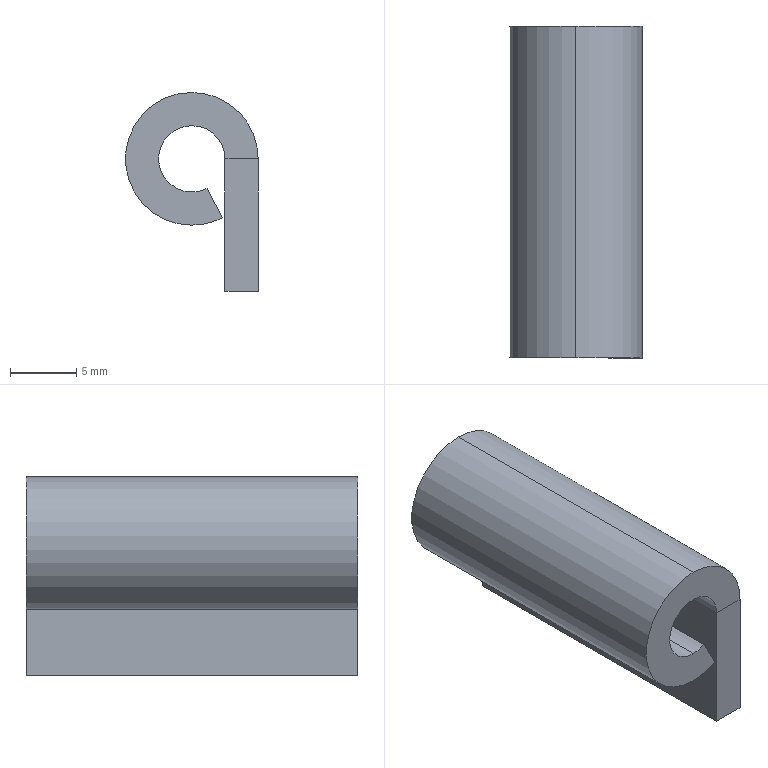Part | SolidWorks | features FlatPattern 1, SMBaseFlange 1, SheetMetal 1 | 1 solid | 14 faces | box 10 x 25 x 15 mm | volume 1841 mm3 | plane 8 | cylinder 6 | commonest cylinder face diameters 5 x3 10 x3
STEP:
#1=CARTESIAN_POINT('',(0.,25.,10.));
#2=VERTEX_POINT('',#1);
#3=CARTESIAN_POINT('',(-5.,25.,15.));
#4=VERTEX_POINT('',#3);
#5=CARTESIAN_POINT('',(-5.,25.,10.));
#6=DIRECTION('',(0.,-1.,0.));
#7=DIRECTION('',(0.,0.,-1.));
#8=AXIS2_PLACEMENT_3D('',#5,#6,#7);
#9=CIRCLE('',#8,5.);
#10=EDGE_CURVE('',#2,#4,#9,.T.);
#11=ORIENTED_EDGE('',*,*,#10,.T.);
#12=CARTESIAN_POINT('',(-5.,0.,15.));
#13=VERTEX_POINT('',#12);
#14=CARTESIAN_POINT('',(-5.,25.,15.));
#15=DIRECTION('',(0.,-1.,0.));
#16=VECTOR('',#15,1000.);
#17=LINE('',#14,#16);
#18=EDGE_CURVE('',#4,#13,#17,.T.);
#19=ORIENTED_EDGE('',*,*,#18,.T.);
#20=CARTESIAN_POINT('',(0.,0.,10.));
#21=VERTEX_POINT('',#20);
#22=CARTESIAN_POINT('',(-5.,0.,10.));
#23=DIRECTION('',(0.,-1.,0.));
#24=DIRECTION('',(0.,0.,-1.));
#25=AXIS2_PLACEMENT_3D('',#22,#23,#24);
#26=CIRCLE('',#25,5.);
#27=EDGE_CURVE('',#21,#13,#26,.T.);
#28=ORIENTED_EDGE('',*,*,#27,.F.);
#29=CARTESIAN_POINT('',(0.,25.,10.));
#30=DIRECTION('',(0.,-1.,0.));
#31=VECTOR('',#30,1000.);
#32=LINE('',#29,#31);
#33=EDGE_CURVE('',#2,#21,#32,.T.);
#34=ORIENTED_EDGE('',*,*,#33,.F.);
#35=EDGE_LOOP('',(#11,#19,#28,#34));
#36=FACE_OUTER_BOUND('',#35,.T.);
#37=CARTESIAN_POINT('',(-5.,25.,10.));
#38=DIRECTION('',(0.,-1.,0.));
#39=DIRECTION('',(0.,0.,-1.));
#40=AXIS2_PLACEMENT_3D('',#37,#38,#39);
#41=CYLINDRICAL_SURFACE('',#40,5.);
#42=ADVANCED_FACE('',(#36),#41,.T.);
#43=ORIENTED_EDGE('',*,*,#18,.F.);
#44=CARTESIAN_POINT('',(-5.,25.,5.));
#45=VERTEX_POINT('',#44);
#46=CARTESIAN_POINT('',(-5.,25.,10.));
#47=DIRECTION('',(0.,-1.,0.));
#48=DIRECTION('',(0.,0.,-1.));
#49=AXIS2_PLACEMENT_3D('',#46,#47,#48);
#50=CIRCLE('',#49,5.);
#51=EDGE_CURVE('',#4,#45,#50,.T.);
#52=ORIENTED_EDGE('',*,*,#51,.T.);
#53=CARTESIAN_POINT('',(-5.,0.,5.));
#54=VERTEX_POINT('',#53);
#55=CARTESIAN_POINT('',(-5.,25.,5.));
#56=DIRECTION('',(0.,-1.,0.));
#57=VECTOR('',#56,1000.);
#58=LINE('',#55,#57);
#59=EDGE_CURVE('',#45,#54,#58,.T.);
#60=ORIENTED_EDGE('',*,*,#59,.T.);
#61=CARTESIAN_POINT('',(-5.,0.,10.));
#62=DIRECTION('',(0.,-1.,0.));
#63=DIRECTION('',(0.,0.,-1.));
#64=AXIS2_PLACEMENT_3D('',#61,#62,#63);
#65=CIRCLE('',#64,5.);
#66=EDGE_CURVE('',#13,#54,#65,.T.);
#67=ORIENTED_EDGE('',*,*,#66,.F.);
#68=EDGE_LOOP('',(#43,#52,#60,#67));
#69=FACE_OUTER_BOUND('',#68,.T.);
#70=CARTESIAN_POINT('',(-5.,25.,10.));
#71=DIRECTION('',(0.,-1.,0.));
#72=DIRECTION('',(0.,0.,-1.));
#73=AXIS2_PLACEMENT_3D('',#70,#71,#72);
#74=CYLINDRICAL_SURFACE('',#73,5.);
#75=ADVANCED_FACE('',(#69),#74,.T.);
#76=CARTESIAN_POINT('',(-5.,25.,12.5));
#77=VERTEX_POINT('',#76);
#78=CARTESIAN_POINT('',(-5.,25.,7.5));
#79=VERTEX_POINT('',#78);
#80=CARTESIAN_POINT('',(-5.,25.,10.));
#81=DIRECTION('',(0.,-1.,0.));
#82=DIRECTION('',(1.,0.,0.));
#83=AXIS2_PLACEMENT_3D('',#80,#81,#82);
#84=CIRCLE('',#83,2.5);
#85=EDGE_CURVE('',#77,#79,#84,.T.);
#86=ORIENTED_EDGE('',*,*,#85,.F.);
#87=CARTESIAN_POINT('',(-5.,0.,12.5));
#88=VERTEX_POINT('',#87);
#89=CARTESIAN_POINT('',(-5.,25.,12.5));
#90=DIRECTION('',(0.,-1.,0.));
#91=VECTOR('',#90,1000.);
#92=LINE('',#89,#91);
#93=EDGE_CURVE('',#77,#88,#92,.T.);
#94=ORIENTED_EDGE('',*,*,#93,.T.);
#95=CARTESIAN_POINT('',(-5.,0.,7.5));
#96=VERTEX_POINT('',#95);
#97=CARTESIAN_POINT('',(-5.,0.,10.));
#98=DIRECTION('',(0.,-1.,0.));
#99=DIRECTION('',(1.,0.,0.));
#100=AXIS2_PLACEMENT_3D('',#97,#98,#99);
#101=CIRCLE('',#100,2.5);
#102=EDGE_CURVE('',#88,#96,#101,.T.);
#103=ORIENTED_EDGE('',*,*,#102,.T.);
#104=CARTESIAN_POINT('',(-5.,25.,7.5));
#105=DIRECTION('',(0.,-1.,0.));
#106=VECTOR('',#105,1000.);
#107=LINE('',#104,#106);
#108=EDGE_CURVE('',#79,#96,#107,.T.);
#109=ORIENTED_EDGE('',*,*,#108,.F.);
#110=EDGE_LOOP('',(#86,#94,#103,#109));
#111=FACE_OUTER_BOUND('',#110,.T.);
#112=CARTESIAN_POINT('',(-5.,25.,10.));
#113=DIRECTION('',(0.,-1.,0.));
#114=DIRECTION('',(0.,0.,-1.));
#115=AXIS2_PLACEMENT_3D('',#112,#113,#114);
#116=CYLINDRICAL_SURFACE('',#115,2.5);
#117=ADVANCED_FACE('',(#111),#116,.F.);
#118=CARTESIAN_POINT('',(-3.85,25.,7.78));
#119=VERTEX_POINT('',#118);
#120=CARTESIAN_POINT('',(-5.,25.,10.));
#121=DIRECTION('',(0.,-1.,0.));
#122=DIRECTION('',(1.,0.,0.));
#123=AXIS2_PLACEMENT_3D('',#120,#121,#122);
#124=CIRCLE('',#123,2.5);
#125=EDGE_CURVE('',#79,#119,#124,.T.);
#126=ORIENTED_EDGE('',*,*,#125,.F.);
#127=ORIENTED_EDGE('',*,*,#108,.T.);
#128=CARTESIAN_POINT('',(-3.85,0.,7.78));
#129=VERTEX_POINT('',#128);
#130=CARTESIAN_POINT('',(-5.,0.,10.));
#131=DIRECTION('',(0.,-1.,0.));
#132=DIRECTION('',(1.,0.,0.));
#133=AXIS2_PLACEMENT_3D('',#130,#131,#132);
#134=CIRCLE('',#133,2.5);
#135=EDGE_CURVE('',#96,#129,#134,.T.);
#136=ORIENTED_EDGE('',*,*,#135,.T.);
#137=CARTESIAN_POINT('',(-3.85,25.,7.78));
#138=DIRECTION('',(0.,-1.,0.));
#139=VECTOR('',#138,1000.);
#140=LINE('',#137,#139);
#141=EDGE_CURVE('',#119,#129,#140,.T.);
#142=ORIENTED_EDGE('',*,*,#141,.F.);
#143=EDGE_LOOP('',(#126,#127,#136,#142));
#144=FACE_OUTER_BOUND('',#143,.T.);
#145=CARTESIAN_POINT('',(-5.,25.,10.));
#146=DIRECTION('',(0.,-1.,0.));
#147=DIRECTION('',(0.,0.,-1.));
#148=AXIS2_PLACEMENT_3D('',#145,#146,#147);
#149=CYLINDRICAL_SURFACE('',#148,2.5);
#150=ADVANCED_FACE('',(#144),#149,.F.);
#151=CARTESIAN_POINT('',(-2.5,25.,10.));
#152=VERTEX_POINT('',#151);
#153=CARTESIAN_POINT('',(-2.5,25.,10.));
#154=DIRECTION('',(1.,0.,0.));
#155=VECTOR('',#154,1000.);
#156=LINE('',#153,#155);
#157=EDGE_CURVE('',#152,#2,#156,.T.);
#158=ORIENTED_EDGE('',*,*,#157,.F.);
#159=CARTESIAN_POINT('',(-5.,25.,10.));
#160=DIRECTION('',(0.,-1.,0.));
#161=DIRECTION('',(1.,0.,0.));
#162=AXIS2_PLACEMENT_3D('',#159,#160,#161);
#163=CIRCLE('',#162,2.5);
#164=EDGE_CURVE('',#152,#77,#163,.T.);
#165=ORIENTED_EDGE('',*,*,#164,.T.);
#166=ORIENTED_EDGE('',*,*,#85,.T.);
#167=ORIENTED_EDGE('',*,*,#125,.T.);
#168=CARTESIAN_POINT('',(-2.7,25.,5.56));
#169=VERTEX_POINT('',#168);
#170=CARTESIAN_POINT('',(-2.7,25.,5.56));
#171=DIRECTION('',(-0.46,0.,0.8879));
#172=VECTOR('',#171,1000.);
#173=LINE('',#170,#172);
#174=EDGE_CURVE('',#169,#119,#173,.T.);
#175=ORIENTED_EDGE('',*,*,#174,.F.);
#176=CARTESIAN_POINT('',(-5.,25.,10.));
#177=DIRECTION('',(0.,-1.,0.));
#178=DIRECTION('',(0.,0.,-1.));
#179=AXIS2_PLACEMENT_3D('',#176,#177,#178);
#180=CIRCLE('',#179,5.);
#181=EDGE_CURVE('',#45,#169,#180,.T.);
#182=ORIENTED_EDGE('',*,*,#181,.F.);
#183=ORIENTED_EDGE('',*,*,#51,.F.);
#184=ORIENTED_EDGE('',*,*,#10,.F.);
#185=EDGE_LOOP('',(#158,#165,#166,#167,#175,#182,#183,#184));
#186=FACE_OUTER_BOUND('',#185,.T.);
#187=CARTESIAN_POINT('',(-2.5,25.,10.));
#188=DIRECTION('',(0.,1.,0.));
#189=DIRECTION('',(0.,0.,1.));
#190=AXIS2_PLACEMENT_3D('',#187,#188,#189);
#191=PLANE('',#190);
#192=ADVANCED_FACE('',(#186),#191,.T.);
#193=CARTESIAN_POINT('',(-2.5,0.,10.));
#194=VERTEX_POINT('',#193);
#195=CARTESIAN_POINT('',(0.,0.,10.));
#196=DIRECTION('',(-1.,0.,0.));
#197=VECTOR('',#196,1000.);
#198=LINE('',#195,#197);
#199=EDGE_CURVE('',#21,#194,#198,.T.);
#200=ORIENTED_EDGE('',*,*,#199,.F.);
#201=ORIENTED_EDGE('',*,*,#27,.T.);
#202=ORIENTED_EDGE('',*,*,#66,.T.);
#203=CARTESIAN_POINT('',(-2.7,0.,5.56));
#204=VERTEX_POINT('',#203);
#205=CARTESIAN_POINT('',(-5.,0.,10.));
#206=DIRECTION('',(0.,-1.,0.));
#207=DIRECTION('',(0.,0.,-1.));
#208=AXIS2_PLACEMENT_3D('',#205,#206,#207);
#209=CIRCLE('',#208,5.);
#210=EDGE_CURVE('',#54,#204,#209,.T.);
#211=ORIENTED_EDGE('',*,*,#210,.T.);
#212=CARTESIAN_POINT('',(-2.7,0.,5.56));
#213=DIRECTION('',(-0.46,0.,0.8879));
#214=VECTOR('',#213,1000.);
#215=LINE('',#212,#214);
#216=EDGE_CURVE('',#204,#129,#215,.T.);
#217=ORIENTED_EDGE('',*,*,#216,.T.);
#218=ORIENTED_EDGE('',*,*,#135,.F.);
#219=ORIENTED_EDGE('',*,*,#102,.F.);
#220=CARTESIAN_POINT('',(-5.,0.,10.));
#221=DIRECTION('',(0.,-1.,0.));
#222=DIRECTION('',(1.,0.,0.));
#223=AXIS2_PLACEMENT_3D('',#220,#221,#222);
#224=CIRCLE('',#223,2.5);
#225=EDGE_CURVE('',#194,#88,#224,.T.);
#226=ORIENTED_EDGE('',*,*,#225,.F.);
#227=EDGE_LOOP('',(#200,#201,#202,#211,#217,#218,#219,#226));
#228=FACE_OUTER_BOUND('',#227,.T.);
#229=CARTESIAN_POINT('',(0.,0.,10.));
#230=DIRECTION('',(0.,-1.,0.));
#231=DIRECTION('',(0.,0.,-1.));
#232=AXIS2_PLACEMENT_3D('',#229,#230,#231);
#233=PLANE('',#232);
#234=ADVANCED_FACE('',(#228),#233,.T.);
#235=ORIENTED_EDGE('',*,*,#93,.F.);
#236=ORIENTED_EDGE('',*,*,#164,.F.);
#237=CARTESIAN_POINT('',(-2.5,25.,10.));
#238=DIRECTION('',(0.,-1.,0.));
#239=VECTOR('',#238,1000.);
#240=LINE('',#237,#239);
#241=EDGE_CURVE('',#152,#194,#240,.T.);
#242=ORIENTED_EDGE('',*,*,#241,.T.);
#243=ORIENTED_EDGE('',*,*,#225,.T.);
#244=EDGE_LOOP('',(#235,#236,#242,#243));
#245=FACE_OUTER_BOUND('',#244,.T.);
#246=CARTESIAN_POINT('',(-5.,25.,10.));
#247=DIRECTION('',(0.,-1.,0.));
#248=DIRECTION('',(0.,0.,-1.));
#249=AXIS2_PLACEMENT_3D('',#246,#247,#248);
#250=CYLINDRICAL_SURFACE('',#249,2.5);
#251=ADVANCED_FACE('',(#245),#250,.F.);
#252=ORIENTED_EDGE('',*,*,#216,.F.);
#253=CARTESIAN_POINT('',(-2.7,25.,5.56));
#254=DIRECTION('',(0.,-1.,0.));
#255=VECTOR('',#254,1000.);
#256=LINE('',#253,#255);
#257=EDGE_CURVE('',#169,#204,#256,.T.);
#258=ORIENTED_EDGE('',*,*,#257,.F.);
#259=ORIENTED_EDGE('',*,*,#174,.T.);
#260=ORIENTED_EDGE('',*,*,#141,.T.);
#261=EDGE_LOOP('',(#252,#258,#259,#260));
#262=FACE_OUTER_BOUND('',#261,.T.);
#263=CARTESIAN_POINT('',(-2.7,25.,5.56));
#264=DIRECTION('',(0.8879,0.,0.46));
#265=DIRECTION('',(0.46,0.,-0.8879));
#266=AXIS2_PLACEMENT_3D('',#263,#264,#265);
#267=PLANE('',#266);
#268=ADVANCED_FACE('',(#262),#267,.T.);
#269=ORIENTED_EDGE('',*,*,#59,.F.);
#270=ORIENTED_EDGE('',*,*,#181,.T.);
#271=ORIENTED_EDGE('',*,*,#257,.T.);
#272=ORIENTED_EDGE('',*,*,#210,.F.);
#273=EDGE_LOOP('',(#269,#270,#271,#272));
#274=FACE_OUTER_BOUND('',#273,.T.);
#275=CARTESIAN_POINT('',(-5.,25.,10.));
#276=DIRECTION('',(0.,-1.,0.));
#277=DIRECTION('',(0.,0.,-1.));
#278=AXIS2_PLACEMENT_3D('',#275,#276,#277);
#279=CYLINDRICAL_SURFACE('',#278,5.);
#280=ADVANCED_FACE('',(#274),#279,.T.);
#281=CARTESIAN_POINT('',(0.,0.,0.));
#282=VERTEX_POINT('',#281);
#283=CARTESIAN_POINT('',(0.,0.,0.));
#284=DIRECTION('',(0.,0.,1.));
#285=VECTOR('',#284,1000.);
#286=LINE('',#283,#285);
#287=EDGE_CURVE('',#282,#21,#286,.T.);
#288=ORIENTED_EDGE('',*,*,#287,.F.);
#289=CARTESIAN_POINT('',(0.,25.,0.));
#290=VERTEX_POINT('',#289);
#291=CARTESIAN_POINT('',(0.,25.,0.));
#292=DIRECTION('',(0.,-1.,0.));
#293=VECTOR('',#292,1000.);
#294=LINE('',#291,#293);
#295=EDGE_CURVE('',#290,#282,#294,.T.);
#296=ORIENTED_EDGE('',*,*,#295,.F.);
#297=CARTESIAN_POINT('',(0.,25.,0.));
#298=DIRECTION('',(0.,0.,1.));
#299=VECTOR('',#298,1000.);
#300=LINE('',#297,#299);
#301=EDGE_CURVE('',#290,#2,#300,.T.);
#302=ORIENTED_EDGE('',*,*,#301,.T.);
#303=ORIENTED_EDGE('',*,*,#33,.T.);
#304=EDGE_LOOP('',(#288,#296,#302,#303));
#305=FACE_OUTER_BOUND('',#304,.T.);
#306=CARTESIAN_POINT('',(0.,25.,0.));
#307=DIRECTION('',(1.,0.,0.));
#308=DIRECTION('',(0.,0.,-1.));
#309=AXIS2_PLACEMENT_3D('',#306,#307,#308);
#310=PLANE('',#309);
#311=ADVANCED_FACE('',(#305),#310,.T.);
#312=CARTESIAN_POINT('',(-2.5,0.,0.));
#313=VERTEX_POINT('',#312);
#314=CARTESIAN_POINT('',(-2.5,0.,0.));
#315=DIRECTION('',(1.,0.,0.));
#316=VECTOR('',#315,1000.);
#317=LINE('',#314,#316);
#318=EDGE_CURVE('',#313,#282,#317,.T.);
#319=ORIENTED_EDGE('',*,*,#318,.F.);
#320=CARTESIAN_POINT('',(-2.5,25.,0.));
#321=VERTEX_POINT('',#320);
#322=CARTESIAN_POINT('',(-2.5,25.,0.));
#323=DIRECTION('',(0.,-1.,0.));
#324=VECTOR('',#323,1000.);
#325=LINE('',#322,#324);
#326=EDGE_CURVE('',#321,#313,#325,.T.);
#327=ORIENTED_EDGE('',*,*,#326,.F.);
#328=CARTESIAN_POINT('',(-2.5,25.,0.));
#329=DIRECTION('',(1.,0.,0.));
#330=VECTOR('',#329,1000.);
#331=LINE('',#328,#330);
#332=EDGE_CURVE('',#321,#290,#331,.T.);
#333=ORIENTED_EDGE('',*,*,#332,.T.);
#334=ORIENTED_EDGE('',*,*,#295,.T.);
#335=EDGE_LOOP('',(#319,#327,#333,#334));
#336=FACE_OUTER_BOUND('',#335,.T.);
#337=CARTESIAN_POINT('',(-2.5,25.,0.));
#338=DIRECTION('',(0.,0.,-1.));
#339=DIRECTION('',(-1.,0.,0.));
#340=AXIS2_PLACEMENT_3D('',#337,#338,#339);
#341=PLANE('',#340);
#342=ADVANCED_FACE('',(#336),#341,.T.);
#343=CARTESIAN_POINT('',(-2.5,0.,0.));
#344=DIRECTION('',(0.,0.,1.));
#345=VECTOR('',#344,1000.);
#346=LINE('',#343,#345);
#347=EDGE_CURVE('',#313,#194,#346,.T.);
#348=ORIENTED_EDGE('',*,*,#347,.T.);
#349=ORIENTED_EDGE('',*,*,#241,.F.);
#350=CARTESIAN_POINT('',(-2.5,25.,0.));
#351=DIRECTION('',(0.,0.,1.));
#352=VECTOR('',#351,1000.);
#353=LINE('',#350,#352);
#354=EDGE_CURVE('',#321,#152,#353,.T.);
#355=ORIENTED_EDGE('',*,*,#354,.F.);
#356=ORIENTED_EDGE('',*,*,#326,.T.);
#357=EDGE_LOOP('',(#348,#349,#355,#356));
#358=FACE_OUTER_BOUND('',#357,.T.);
#359=CARTESIAN_POINT('',(-2.5,25.,0.));
#360=DIRECTION('',(1.,0.,0.));
#361=DIRECTION('',(0.,0.,-1.));
#362=AXIS2_PLACEMENT_3D('',#359,#360,#361);
#363=PLANE('',#362);
#364=ADVANCED_FACE('',(#358),#363,.F.);
#365=ORIENTED_EDGE('',*,*,#354,.T.);
#366=ORIENTED_EDGE('',*,*,#157,.T.);
#367=ORIENTED_EDGE('',*,*,#301,.F.);
#368=ORIENTED_EDGE('',*,*,#332,.F.);
#369=EDGE_LOOP('',(#365,#366,#367,#368));
#370=FACE_OUTER_BOUND('',#369,.T.);
#371=CARTESIAN_POINT('',(-5.,25.,10.));
#372=DIRECTION('',(0.,1.,0.));
#373=DIRECTION('',(0.,0.,1.));
#374=AXIS2_PLACEMENT_3D('',#371,#372,#373);
#375=PLANE('',#374);
#376=ADVANCED_FACE('',(#370),#375,.T.);
#377=ORIENTED_EDGE('',*,*,#287,.T.);
#378=ORIENTED_EDGE('',*,*,#199,.T.);
#379=ORIENTED_EDGE('',*,*,#347,.F.);
#380=ORIENTED_EDGE('',*,*,#318,.T.);
#381=EDGE_LOOP('',(#377,#378,#379,#380));
#382=FACE_OUTER_BOUND('',#381,.T.);
#383=CARTESIAN_POINT('',(-5.,0.,10.));
#384=DIRECTION('',(0.,1.,0.));
#385=DIRECTION('',(0.,0.,1.));
#386=AXIS2_PLACEMENT_3D('',#383,#384,#385);
#387=PLANE('',#386);
#388=ADVANCED_FACE('',(#382),#387,.F.);
#389=CLOSED_SHELL('',(#42,#75,#117,#150,#192,#234,#251,#268,#280,#311,#342,#364,#376,#388));
#390=MANIFOLD_SOLID_BREP('',#389);
#391=CARTESIAN_POINT('',(0.,0.,0.));
#392=DIRECTION('',(0.,0.,1.));
#393=DIRECTION('',(1.,0.,0.));
#394=AXIS2_PLACEMENT_3D('',#391,#392,#393);
#395=(LENGTH_UNIT()NAMED_UNIT(*)SI_UNIT(.MILLI.,.METRE.));
#396=UNCERTAINTY_MEASURE_WITH_UNIT(LENGTH_MEASURE(0.00001),#395,'','');
#397=(NAMED_UNIT(*)PLANE_ANGLE_UNIT()SI_UNIT($,.RADIAN.));
#398=(NAMED_UNIT(*)SI_UNIT($,.STERADIAN.)SOLID_ANGLE_UNIT());
#399=(GEOMETRIC_REPRESENTATION_CONTEXT(3)GLOBAL_UNCERTAINTY_ASSIGNED_CONTEXT((#396))GLOBAL_UNIT_ASSIGNED_CONTEXT((#395,#397,#398))REPRESENTATION_CONTEXT('',''));
#400=ADVANCED_BREP_SHAPE_REPRESENTATION('',(#390,#394),#399);